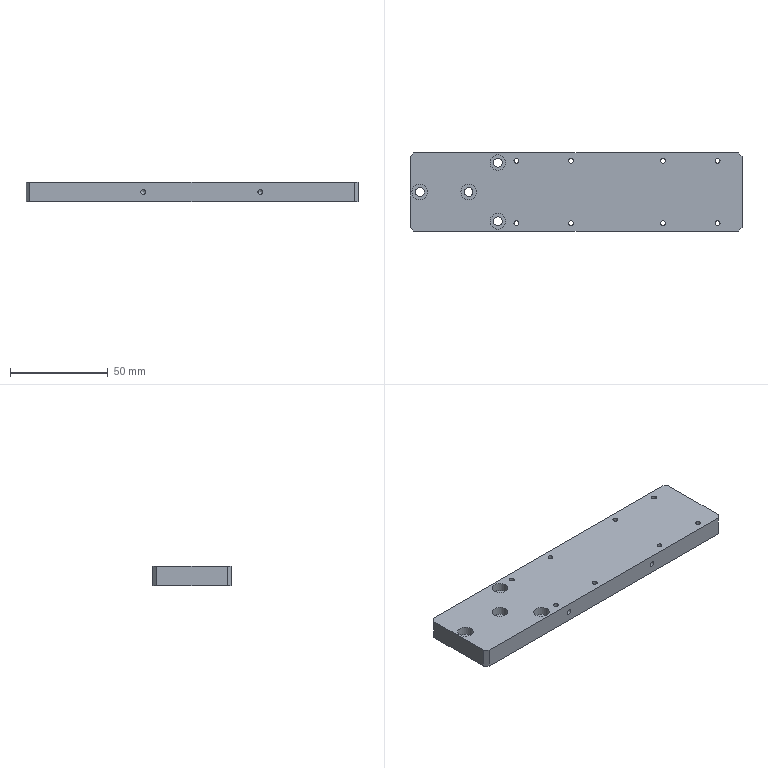Part | NX | 1 solid | 38 faces | box 170 x 40 x 10 mm | volume 66032 mm3 | cylinder 20 | plane 14 | cone 4 | commonest cylinder face diameters 2.5 x10 4.5 x4 8 x4 3.3 x2
STEP:
#1=CARTESIAN_POINT('',(85.,18.,10.));
#2=VERTEX_POINT('',#1);
#3=CARTESIAN_POINT('',(83.,20.,10.));
#4=VERTEX_POINT('',#3);
#5=CARTESIAN_POINT('',(51.5,51.5,10.));
#6=DIRECTION('',(-0.7071,0.7071,0.));
#7=VECTOR('',#6,1000.);
#8=LINE('',#5,#7);
#9=EDGE_CURVE('',#2,#4,#8,.T.);
#10=ORIENTED_EDGE('',*,*,#9,.F.);
#11=CARTESIAN_POINT('',(85.,18.,0.));
#12=VERTEX_POINT('',#11);
#13=CARTESIAN_POINT('',(85.,18.,10.));
#14=DIRECTION('',(0.,0.,1.));
#15=VECTOR('',#14,1000.);
#16=LINE('',#13,#15);
#17=EDGE_CURVE('',#12,#2,#16,.T.);
#18=ORIENTED_EDGE('',*,*,#17,.F.);
#19=CARTESIAN_POINT('',(83.,20.,0.));
#20=VERTEX_POINT('',#19);
#21=CARTESIAN_POINT('',(83.,20.,0.));
#22=DIRECTION('',(0.7071,-0.7071,0.));
#23=VECTOR('',#22,1000.);
#24=LINE('',#21,#23);
#25=EDGE_CURVE('',#20,#12,#24,.T.);
#26=ORIENTED_EDGE('',*,*,#25,.F.);
#27=CARTESIAN_POINT('',(83.,20.,10.));
#28=DIRECTION('',(0.,0.,-1.));
#29=VECTOR('',#28,1000.);
#30=LINE('',#27,#29);
#31=EDGE_CURVE('',#4,#20,#30,.T.);
#32=ORIENTED_EDGE('',*,*,#31,.F.);
#33=EDGE_LOOP('',(#10,#18,#26,#32));
#34=FACE_BOUND('',#33,.T.);
#35=CARTESIAN_POINT('',(83.,20.,10.));
#36=DIRECTION('',(-0.7071,-0.7071,0.));
#37=DIRECTION('',(0.,0.,-1.));
#38=AXIS2_PLACEMENT_3D('',#35,#36,#37);
#39=PLANE('',#38);
#40=ADVANCED_FACE('',(#34),#39,.F.);
#41=CARTESIAN_POINT('',(83.,-20.,10.));
#42=VERTEX_POINT('',#41);
#43=CARTESIAN_POINT('',(85.,-18.,10.));
#44=VERTEX_POINT('',#43);
#45=CARTESIAN_POINT('',(51.5,-51.5,10.));
#46=DIRECTION('',(0.7071,0.7071,0.));
#47=VECTOR('',#46,1000.);
#48=LINE('',#45,#47);
#49=EDGE_CURVE('',#42,#44,#48,.T.);
#50=ORIENTED_EDGE('',*,*,#49,.F.);
#51=CARTESIAN_POINT('',(83.,-20.,0.));
#52=VERTEX_POINT('',#51);
#53=CARTESIAN_POINT('',(83.,-20.,10.));
#54=DIRECTION('',(0.,0.,1.));
#55=VECTOR('',#54,1000.);
#56=LINE('',#53,#55);
#57=EDGE_CURVE('',#52,#42,#56,.T.);
#58=ORIENTED_EDGE('',*,*,#57,.F.);
#59=CARTESIAN_POINT('',(85.,-18.,0.));
#60=VERTEX_POINT('',#59);
#61=CARTESIAN_POINT('',(85.,-18.,0.));
#62=DIRECTION('',(-0.7071,-0.7071,0.));
#63=VECTOR('',#62,1000.);
#64=LINE('',#61,#63);
#65=EDGE_CURVE('',#60,#52,#64,.T.);
#66=ORIENTED_EDGE('',*,*,#65,.F.);
#67=CARTESIAN_POINT('',(85.,-18.,10.));
#68=DIRECTION('',(0.,0.,-1.));
#69=VECTOR('',#68,1000.);
#70=LINE('',#67,#69);
#71=EDGE_CURVE('',#44,#60,#70,.T.);
#72=ORIENTED_EDGE('',*,*,#71,.F.);
#73=EDGE_LOOP('',(#50,#58,#66,#72));
#74=FACE_BOUND('',#73,.T.);
#75=CARTESIAN_POINT('',(85.,-18.,10.));
#76=DIRECTION('',(-0.7071,0.7071,0.));
#77=DIRECTION('',(0.,0.,-1.));
#78=AXIS2_PLACEMENT_3D('',#75,#76,#77);
#79=PLANE('',#78);
#80=ADVANCED_FACE('',(#74),#79,.F.);
#81=CARTESIAN_POINT('',(-85.,-18.,10.));
#82=VERTEX_POINT('',#81);
#83=CARTESIAN_POINT('',(-83.,-20.,10.));
#84=VERTEX_POINT('',#83);
#85=CARTESIAN_POINT('',(-51.5,-51.5,10.));
#86=DIRECTION('',(0.7071,-0.7071,0.));
#87=VECTOR('',#86,1000.);
#88=LINE('',#85,#87);
#89=EDGE_CURVE('',#82,#84,#88,.T.);
#90=ORIENTED_EDGE('',*,*,#89,.F.);
#91=CARTESIAN_POINT('',(-85.,-18.,0.));
#92=VERTEX_POINT('',#91);
#93=CARTESIAN_POINT('',(-85.,-18.,10.));
#94=DIRECTION('',(0.,0.,1.));
#95=VECTOR('',#94,1000.);
#96=LINE('',#93,#95);
#97=EDGE_CURVE('',#92,#82,#96,.T.);
#98=ORIENTED_EDGE('',*,*,#97,.F.);
#99=CARTESIAN_POINT('',(-83.,-20.,0.));
#100=VERTEX_POINT('',#99);
#101=CARTESIAN_POINT('',(-83.,-20.,0.));
#102=DIRECTION('',(-0.7071,0.7071,0.));
#103=VECTOR('',#102,1000.);
#104=LINE('',#101,#103);
#105=EDGE_CURVE('',#100,#92,#104,.T.);
#106=ORIENTED_EDGE('',*,*,#105,.F.);
#107=CARTESIAN_POINT('',(-83.,-20.,10.));
#108=DIRECTION('',(0.,0.,-1.));
#109=VECTOR('',#108,1000.);
#110=LINE('',#107,#109);
#111=EDGE_CURVE('',#84,#100,#110,.T.);
#112=ORIENTED_EDGE('',*,*,#111,.F.);
#113=EDGE_LOOP('',(#90,#98,#106,#112));
#114=FACE_BOUND('',#113,.T.);
#115=CARTESIAN_POINT('',(-83.,-20.,10.));
#116=DIRECTION('',(0.7071,0.7071,0.));
#117=DIRECTION('',(0.,0.,-1.));
#118=AXIS2_PLACEMENT_3D('',#115,#116,#117);
#119=PLANE('',#118);
#120=ADVANCED_FACE('',(#114),#119,.F.);
#121=CARTESIAN_POINT('',(-83.,20.,10.));
#122=VERTEX_POINT('',#121);
#123=CARTESIAN_POINT('',(-85.,18.,10.));
#124=VERTEX_POINT('',#123);
#125=CARTESIAN_POINT('',(-51.5,51.5,10.));
#126=DIRECTION('',(-0.7071,-0.7071,0.));
#127=VECTOR('',#126,1000.);
#128=LINE('',#125,#127);
#129=EDGE_CURVE('',#122,#124,#128,.T.);
#130=ORIENTED_EDGE('',*,*,#129,.F.);
#131=CARTESIAN_POINT('',(-83.,20.,0.));
#132=VERTEX_POINT('',#131);
#133=CARTESIAN_POINT('',(-83.,20.,10.));
#134=DIRECTION('',(0.,0.,1.));
#135=VECTOR('',#134,1000.);
#136=LINE('',#133,#135);
#137=EDGE_CURVE('',#132,#122,#136,.T.);
#138=ORIENTED_EDGE('',*,*,#137,.F.);
#139=CARTESIAN_POINT('',(-85.,18.,0.));
#140=VERTEX_POINT('',#139);
#141=CARTESIAN_POINT('',(-85.,18.,0.));
#142=DIRECTION('',(0.7071,0.7071,0.));
#143=VECTOR('',#142,1000.);
#144=LINE('',#141,#143);
#145=EDGE_CURVE('',#140,#132,#144,.T.);
#146=ORIENTED_EDGE('',*,*,#145,.F.);
#147=CARTESIAN_POINT('',(-85.,18.,10.));
#148=DIRECTION('',(0.,0.,-1.));
#149=VECTOR('',#148,1000.);
#150=LINE('',#147,#149);
#151=EDGE_CURVE('',#124,#140,#150,.T.);
#152=ORIENTED_EDGE('',*,*,#151,.F.);
#153=EDGE_LOOP('',(#130,#138,#146,#152));
#154=FACE_BOUND('',#153,.T.);
#155=CARTESIAN_POINT('',(-85.,18.,10.));
#156=DIRECTION('',(0.7071,-0.7071,0.));
#157=DIRECTION('',(0.,0.,-1.));
#158=AXIS2_PLACEMENT_3D('',#155,#156,#157);
#159=PLANE('',#158);
#160=ADVANCED_FACE('',(#154),#159,.F.);
#161=CARTESIAN_POINT('',(-59.,0.,5.6));
#162=VERTEX_POINT('',#161);
#163=CARTESIAN_POINT('',(-55.,0.,5.6));
#164=DIRECTION('',(0.,0.,1.));
#165=DIRECTION('',(-1.,0.,0.));
#166=AXIS2_PLACEMENT_3D('',#163,#164,#165);
#167=CIRCLE('',#166,4.);
#168=EDGE_CURVE('',#162,#162,#167,.T.);
#169=ORIENTED_EDGE('',*,*,#168,.T.);
#170=EDGE_LOOP('',(#169));
#171=FACE_BOUND('',#170,.T.);
#172=CARTESIAN_POINT('',(-57.25,0.,5.6));
#173=VERTEX_POINT('',#172);
#174=CARTESIAN_POINT('',(-55.,0.,5.6));
#175=DIRECTION('',(0.,0.,1.));
#176=DIRECTION('',(-1.,0.,0.));
#177=AXIS2_PLACEMENT_3D('',#174,#175,#176);
#178=CIRCLE('',#177,2.25);
#179=EDGE_CURVE('',#173,#173,#178,.T.);
#180=ORIENTED_EDGE('',*,*,#179,.F.);
#181=EDGE_LOOP('',(#180));
#182=FACE_BOUND('',#181,.T.);
#183=CARTESIAN_POINT('',(-77.75,0.,5.6));
#184=DIRECTION('',(0.,0.,-1.));
#185=DIRECTION('',(-1.,0.,0.));
#186=AXIS2_PLACEMENT_3D('',#183,#184,#185);
#187=PLANE('',#186);
#188=ADVANCED_FACE('',(#171,#182),#187,.F.);
#189=CARTESIAN_POINT('',(-76.,0.,5.6));
#190=VERTEX_POINT('',#189);
#191=CARTESIAN_POINT('',(-80.,0.,5.6));
#192=DIRECTION('',(0.,0.,1.));
#193=DIRECTION('',(1.,0.,0.));
#194=AXIS2_PLACEMENT_3D('',#191,#192,#193);
#195=CIRCLE('',#194,4.);
#196=EDGE_CURVE('',#190,#190,#195,.T.);
#197=ORIENTED_EDGE('',*,*,#196,.T.);
#198=EDGE_LOOP('',(#197));
#199=FACE_BOUND('',#198,.T.);
#200=CARTESIAN_POINT('',(-77.75,0.,5.6));
#201=VERTEX_POINT('',#200);
#202=CARTESIAN_POINT('',(-80.,0.,5.6));
#203=DIRECTION('',(0.,0.,1.));
#204=DIRECTION('',(1.,0.,0.));
#205=AXIS2_PLACEMENT_3D('',#202,#203,#204);
#206=CIRCLE('',#205,2.25);
#207=EDGE_CURVE('',#201,#201,#206,.T.);
#208=ORIENTED_EDGE('',*,*,#207,.F.);
#209=EDGE_LOOP('',(#208));
#210=FACE_BOUND('',#209,.T.);
#211=CARTESIAN_POINT('',(-77.75,0.,5.6));
#212=DIRECTION('',(0.,0.,-1.));
#213=DIRECTION('',(-1.,0.,0.));
#214=AXIS2_PLACEMENT_3D('',#211,#212,#213);
#215=PLANE('',#214);
#216=ADVANCED_FACE('',(#199,#210),#215,.F.);
#217=CARTESIAN_POINT('',(-44.,15.,5.6));
#218=VERTEX_POINT('',#217);
#219=CARTESIAN_POINT('',(-40.,15.,5.6));
#220=DIRECTION('',(0.,0.,1.));
#221=DIRECTION('',(-1.,0.,0.));
#222=AXIS2_PLACEMENT_3D('',#219,#220,#221);
#223=CIRCLE('',#222,4.);
#224=EDGE_CURVE('',#218,#218,#223,.T.);
#225=ORIENTED_EDGE('',*,*,#224,.T.);
#226=EDGE_LOOP('',(#225));
#227=FACE_BOUND('',#226,.T.);
#228=CARTESIAN_POINT('',(-42.25,15.,5.6));
#229=VERTEX_POINT('',#228);
#230=CARTESIAN_POINT('',(-40.,15.,5.6));
#231=DIRECTION('',(0.,0.,1.));
#232=DIRECTION('',(-1.,0.,0.));
#233=AXIS2_PLACEMENT_3D('',#230,#231,#232);
#234=CIRCLE('',#233,2.25);
#235=EDGE_CURVE('',#229,#229,#234,.T.);
#236=ORIENTED_EDGE('',*,*,#235,.F.);
#237=EDGE_LOOP('',(#236));
#238=FACE_BOUND('',#237,.T.);
#239=CARTESIAN_POINT('',(-77.75,0.,5.6));
#240=DIRECTION('',(0.,0.,-1.));
#241=DIRECTION('',(-1.,0.,0.));
#242=AXIS2_PLACEMENT_3D('',#239,#240,#241);
#243=PLANE('',#242);
#244=ADVANCED_FACE('',(#227,#238),#243,.F.);
#245=CARTESIAN_POINT('',(-44.,-15.,5.6));
#246=VERTEX_POINT('',#245);
#247=CARTESIAN_POINT('',(-40.,-15.,5.6));
#248=DIRECTION('',(0.,0.,1.));
#249=DIRECTION('',(-1.,0.,0.));
#250=AXIS2_PLACEMENT_3D('',#247,#248,#249);
#251=CIRCLE('',#250,4.);
#252=EDGE_CURVE('',#246,#246,#251,.T.);
#253=ORIENTED_EDGE('',*,*,#252,.T.);
#254=EDGE_LOOP('',(#253));
#255=FACE_BOUND('',#254,.T.);
#256=CARTESIAN_POINT('',(-42.25,-15.,5.6));
#257=VERTEX_POINT('',#256);
#258=CARTESIAN_POINT('',(-40.,-15.,5.6));
#259=DIRECTION('',(0.,0.,1.));
#260=DIRECTION('',(-1.,0.,0.));
#261=AXIS2_PLACEMENT_3D('',#258,#259,#260);
#262=CIRCLE('',#261,2.25);
#263=EDGE_CURVE('',#257,#257,#262,.T.);
#264=ORIENTED_EDGE('',*,*,#263,.F.);
#265=EDGE_LOOP('',(#264));
#266=FACE_BOUND('',#265,.T.);
#267=CARTESIAN_POINT('',(-77.75,0.,5.6));
#268=DIRECTION('',(0.,0.,-1.));
#269=DIRECTION('',(-1.,0.,0.));
#270=AXIS2_PLACEMENT_3D('',#267,#268,#269);
#271=PLANE('',#270);
#272=ADVANCED_FACE('',(#255,#266),#271,.F.);
#273=CARTESIAN_POINT('',(-85.,20.,0.));
#274=DIRECTION('',(0.,-1.,0.));
#275=VECTOR('',#274,1000.);
#276=LINE('',#273,#275);
#277=EDGE_CURVE('',#140,#92,#276,.T.);
#278=ORIENTED_EDGE('',*,*,#277,.F.);
#279=ORIENTED_EDGE('',*,*,#145,.T.);
#280=CARTESIAN_POINT('',(-85.,20.,0.));
#281=DIRECTION('',(-1.,0.,0.));
#282=VECTOR('',#281,1000.);
#283=LINE('',#280,#282);
#284=EDGE_CURVE('',#20,#132,#283,.T.);
#285=ORIENTED_EDGE('',*,*,#284,.F.);
#286=ORIENTED_EDGE('',*,*,#25,.T.);
#287=CARTESIAN_POINT('',(85.,20.,0.));
#288=DIRECTION('',(0.,1.,0.));
#289=VECTOR('',#288,1000.);
#290=LINE('',#287,#289);
#291=EDGE_CURVE('',#60,#12,#290,.T.);
#292=ORIENTED_EDGE('',*,*,#291,.F.);
#293=ORIENTED_EDGE('',*,*,#65,.T.);
#294=CARTESIAN_POINT('',(-85.,-20.,0.));
#295=DIRECTION('',(1.,0.,0.));
#296=VECTOR('',#295,1000.);
#297=LINE('',#294,#296);
#298=EDGE_CURVE('',#100,#52,#297,.T.);
#299=ORIENTED_EDGE('',*,*,#298,.F.);
#300=ORIENTED_EDGE('',*,*,#105,.T.);
#301=EDGE_LOOP('',(#278,#279,#285,#286,#292,#293,#299,#300));
#302=FACE_BOUND('',#301,.T.);
#303=CARTESIAN_POINT('',(45.75,16.,0.));
#304=VERTEX_POINT('',#303);
#305=CARTESIAN_POINT('',(44.5,16.,0.));
#306=DIRECTION('',(0.,0.,1.));
#307=DIRECTION('',(1.,0.,0.));
#308=AXIS2_PLACEMENT_3D('',#305,#306,#307);
#309=CIRCLE('',#308,1.25);
#310=EDGE_CURVE('',#304,#304,#309,.T.);
#311=ORIENTED_EDGE('',*,*,#310,.T.);
#312=EDGE_LOOP('',(#311));
#313=FACE_BOUND('',#312,.T.);
#314=CARTESIAN_POINT('',(-29.25,16.,0.));
#315=VERTEX_POINT('',#314);
#316=CARTESIAN_POINT('',(-30.5,16.,0.));
#317=DIRECTION('',(0.,0.,1.));
#318=DIRECTION('',(1.,0.,0.));
#319=AXIS2_PLACEMENT_3D('',#316,#317,#318);
#320=CIRCLE('',#319,1.25);
#321=EDGE_CURVE('',#315,#315,#320,.T.);
#322=ORIENTED_EDGE('',*,*,#321,.T.);
#323=EDGE_LOOP('',(#322));
#324=FACE_BOUND('',#323,.T.);
#325=CARTESIAN_POINT('',(-29.25,-16.,0.));
#326=VERTEX_POINT('',#325);
#327=CARTESIAN_POINT('',(-30.5,-16.,0.));
#328=DIRECTION('',(0.,0.,1.));
#329=DIRECTION('',(1.,0.,0.));
#330=AXIS2_PLACEMENT_3D('',#327,#328,#329);
#331=CIRCLE('',#330,1.25);
#332=EDGE_CURVE('',#326,#326,#331,.T.);
#333=ORIENTED_EDGE('',*,*,#332,.T.);
#334=EDGE_LOOP('',(#333));
#335=FACE_BOUND('',#334,.T.);
#336=CARTESIAN_POINT('',(45.75,-16.,0.));
#337=VERTEX_POINT('',#336);
#338=CARTESIAN_POINT('',(44.5,-16.,0.));
#339=DIRECTION('',(0.,0.,1.));
#340=DIRECTION('',(1.,0.,0.));
#341=AXIS2_PLACEMENT_3D('',#338,#339,#340);
#342=CIRCLE('',#341,1.25);
#343=EDGE_CURVE('',#337,#337,#342,.T.);
#344=ORIENTED_EDGE('',*,*,#343,.T.);
#345=EDGE_LOOP('',(#344));
#346=FACE_BOUND('',#345,.T.);
#347=CARTESIAN_POINT('',(-1.25,-16.,0.));
#348=VERTEX_POINT('',#347);
#349=CARTESIAN_POINT('',(-2.5,-16.,0.));
#350=DIRECTION('',(0.,0.,1.));
#351=DIRECTION('',(1.,0.,0.));
#352=AXIS2_PLACEMENT_3D('',#349,#350,#351);
#353=CIRCLE('',#352,1.25);
#354=EDGE_CURVE('',#348,#348,#353,.T.);
#355=ORIENTED_EDGE('',*,*,#354,.T.);
#356=EDGE_LOOP('',(#355));
#357=FACE_BOUND('',#356,.T.);
#358=CARTESIAN_POINT('',(-1.25,16.,0.));
#359=VERTEX_POINT('',#358);
#360=CARTESIAN_POINT('',(-2.5,16.,0.));
#361=DIRECTION('',(0.,0.,1.));
#362=DIRECTION('',(1.,0.,0.));
#363=AXIS2_PLACEMENT_3D('',#360,#361,#362);
#364=CIRCLE('',#363,1.25);
#365=EDGE_CURVE('',#359,#359,#364,.T.);
#366=ORIENTED_EDGE('',*,*,#365,.T.);
#367=EDGE_LOOP('',(#366));
#368=FACE_BOUND('',#367,.T.);
#369=CARTESIAN_POINT('',(73.75,-16.,0.));
#370=VERTEX_POINT('',#369);
#371=CARTESIAN_POINT('',(72.5,-16.,0.));
#372=DIRECTION('',(0.,0.,1.));
#373=DIRECTION('',(1.,0.,0.));
#374=AXIS2_PLACEMENT_3D('',#371,#372,#373);
#375=CIRCLE('',#374,1.25);
#376=EDGE_CURVE('',#370,#370,#375,.T.);
#377=ORIENTED_EDGE('',*,*,#376,.T.);
#378=EDGE_LOOP('',(#377));
#379=FACE_BOUND('',#378,.T.);
#380=CARTESIAN_POINT('',(73.75,16.,0.));
#381=VERTEX_POINT('',#380);
#382=CARTESIAN_POINT('',(72.5,16.,0.));
#383=DIRECTION('',(0.,0.,1.));
#384=DIRECTION('',(1.,0.,0.));
#385=AXIS2_PLACEMENT_3D('',#382,#383,#384);
#386=CIRCLE('',#385,1.25);
#387=EDGE_CURVE('',#381,#381,#386,.T.);
#388=ORIENTED_EDGE('',*,*,#387,.T.);
#389=EDGE_LOOP('',(#388));
#390=FACE_BOUND('',#389,.T.);
#391=CARTESIAN_POINT('',(-37.75,-15.,0.));
#392=VERTEX_POINT('',#391);
#393=CARTESIAN_POINT('',(-40.,-15.,0.));
#394=DIRECTION('',(0.,0.,1.));
#395=DIRECTION('',(1.,0.,0.));
#396=AXIS2_PLACEMENT_3D('',#393,#394,#395);
#397=CIRCLE('',#396,2.25);
#398=EDGE_CURVE('',#392,#392,#397,.T.);
#399=ORIENTED_EDGE('',*,*,#398,.T.);
#400=EDGE_LOOP('',(#399));
#401=FACE_BOUND('',#400,.T.);
#402=CARTESIAN_POINT('',(-37.75,15.,0.));
#403=VERTEX_POINT('',#402);
#404=CARTESIAN_POINT('',(-40.,15.,0.));
#405=DIRECTION('',(0.,0.,1.));
#406=DIRECTION('',(1.,0.,0.));
#407=AXIS2_PLACEMENT_3D('',#404,#405,#406);
#408=CIRCLE('',#407,2.25);
#409=EDGE_CURVE('',#403,#403,#408,.T.);
#410=ORIENTED_EDGE('',*,*,#409,.T.);
#411=EDGE_LOOP('',(#410));
#412=FACE_BOUND('',#411,.T.);
#413=CARTESIAN_POINT('',(-77.75,0.,0.));
#414=VERTEX_POINT('',#413);
#415=CARTESIAN_POINT('',(-80.,0.,0.));
#416=DIRECTION('',(0.,0.,1.));
#417=DIRECTION('',(1.,0.,0.));
#418=AXIS2_PLACEMENT_3D('',#415,#416,#417);
#419=CIRCLE('',#418,2.25);
#420=EDGE_CURVE('',#414,#414,#419,.T.);
#421=ORIENTED_EDGE('',*,*,#420,.T.);
#422=EDGE_LOOP('',(#421));
#423=FACE_BOUND('',#422,.T.);
#424=CARTESIAN_POINT('',(-52.75,0.,0.));
#425=VERTEX_POINT('',#424);
#426=CARTESIAN_POINT('',(-55.,0.,0.));
#427=DIRECTION('',(0.,0.,1.));
#428=DIRECTION('',(1.,0.,0.));
#429=AXIS2_PLACEMENT_3D('',#426,#427,#428);
#430=CIRCLE('',#429,2.25);
#431=EDGE_CURVE('',#425,#425,#430,.T.);
#432=ORIENTED_EDGE('',*,*,#431,.T.);
#433=EDGE_LOOP('',(#432));
#434=FACE_BOUND('',#433,.T.);
#435=CARTESIAN_POINT('',(0.,0.,0.));
#436=DIRECTION('',(0.,0.,1.));
#437=DIRECTION('',(1.,0.,0.));
#438=AXIS2_PLACEMENT_3D('',#435,#436,#437);
#439=PLANE('',#438);
#440=ADVANCED_FACE('',(#302,#313,#324,#335,#346,#357,#368,#379,#390,#401,#412,#423,#434),#439,.F.);
#441=CARTESIAN_POINT('',(-85.,20.,10.));
#442=DIRECTION('',(-1.,0.,0.));
#443=VECTOR('',#442,1000.);
#444=LINE('',#441,#443);
#445=EDGE_CURVE('',#4,#122,#444,.T.);
#446=ORIENTED_EDGE('',*,*,#445,.T.);
#447=ORIENTED_EDGE('',*,*,#129,.T.);
#448=CARTESIAN_POINT('',(-85.,20.,10.));
#449=DIRECTION('',(0.,-1.,0.));
#450=VECTOR('',#449,1000.);
#451=LINE('',#448,#450);
#452=EDGE_CURVE('',#124,#82,#451,.T.);
#453=ORIENTED_EDGE('',*,*,#452,.T.);
#454=ORIENTED_EDGE('',*,*,#89,.T.);
#455=CARTESIAN_POINT('',(-85.,-20.,10.));
#456=DIRECTION('',(1.,0.,0.));
#457=VECTOR('',#456,1000.);
#458=LINE('',#455,#457);
#459=EDGE_CURVE('',#84,#42,#458,.T.);
#460=ORIENTED_EDGE('',*,*,#459,.T.);
#461=ORIENTED_EDGE('',*,*,#49,.T.);
#462=CARTESIAN_POINT('',(85.,20.,10.));
#463=DIRECTION('',(0.,1.,0.));
#464=VECTOR('',#463,1000.);
#465=LINE('',#462,#464);
#466=EDGE_CURVE('',#44,#2,#465,.T.);
#467=ORIENTED_EDGE('',*,*,#466,.T.);
#468=ORIENTED_EDGE('',*,*,#9,.T.);
#469=EDGE_LOOP('',(#446,#447,#453,#454,#460,#461,#467,#468));
#470=FACE_BOUND('',#469,.T.);
#471=CARTESIAN_POINT('',(45.75,16.,10.));
#472=VERTEX_POINT('',#471);
#473=CARTESIAN_POINT('',(44.5,16.,10.));
#474=DIRECTION('',(0.,0.,1.));
#475=DIRECTION('',(1.,0.,0.));
#476=AXIS2_PLACEMENT_3D('',#473,#474,#475);
#477=CIRCLE('',#476,1.25);
#478=EDGE_CURVE('',#472,#472,#477,.T.);
#479=ORIENTED_EDGE('',*,*,#478,.F.);
#480=EDGE_LOOP('',(#479));
#481=FACE_BOUND('',#480,.T.);
#482=CARTESIAN_POINT('',(-29.25,16.,10.));
#483=VERTEX_POINT('',#482);
#484=CARTESIAN_POINT('',(-30.5,16.,10.));
#485=DIRECTION('',(0.,0.,1.));
#486=DIRECTION('',(1.,0.,0.));
#487=AXIS2_PLACEMENT_3D('',#484,#485,#486);
#488=CIRCLE('',#487,1.25);
#489=EDGE_CURVE('',#483,#483,#488,.T.);
#490=ORIENTED_EDGE('',*,*,#489,.F.);
#491=EDGE_LOOP('',(#490));
#492=FACE_BOUND('',#491,.T.);
#493=CARTESIAN_POINT('',(-29.25,-16.,10.));
#494=VERTEX_POINT('',#493);
#495=CARTESIAN_POINT('',(-30.5,-16.,10.));
#496=DIRECTION('',(0.,0.,1.));
#497=DIRECTION('',(1.,0.,0.));
#498=AXIS2_PLACEMENT_3D('',#495,#496,#497);
#499=CIRCLE('',#498,1.25);
#500=EDGE_CURVE('',#494,#494,#499,.T.);
#501=ORIENTED_EDGE('',*,*,#500,.F.);
#502=EDGE_LOOP('',(#501));
#503=FACE_BOUND('',#502,.T.);
#504=CARTESIAN_POINT('',(45.75,-16.,10.));
#505=VERTEX_POINT('',#504);
#506=CARTESIAN_POINT('',(44.5,-16.,10.));
#507=DIRECTION('',(0.,0.,1.));
#508=DIRECTION('',(1.,0.,0.));
#509=AXIS2_PLACEMENT_3D('',#506,#507,#508);
#510=CIRCLE('',#509,1.25);
#511=EDGE_CURVE('',#505,#505,#510,.T.);
#512=ORIENTED_EDGE('',*,*,#511,.F.);
#513=EDGE_LOOP('',(#512));
#514=FACE_BOUND('',#513,.T.);
#515=CARTESIAN_POINT('',(-1.25,-16.,10.));
#516=VERTEX_POINT('',#515);
#517=CARTESIAN_POINT('',(-2.5,-16.,10.));
#518=DIRECTION('',(0.,0.,1.));
#519=DIRECTION('',(1.,0.,0.));
#520=AXIS2_PLACEMENT_3D('',#517,#518,#519);
#521=CIRCLE('',#520,1.25);
#522=EDGE_CURVE('',#516,#516,#521,.T.);
#523=ORIENTED_EDGE('',*,*,#522,.F.);
#524=EDGE_LOOP('',(#523));
#525=FACE_BOUND('',#524,.T.);
#526=CARTESIAN_POINT('',(-1.25,16.,10.));
#527=VERTEX_POINT('',#526);
#528=CARTESIAN_POINT('',(-2.5,16.,10.));
#529=DIRECTION('',(0.,0.,1.));
#530=DIRECTION('',(1.,0.,0.));
#531=AXIS2_PLACEMENT_3D('',#528,#529,#530);
#532=CIRCLE('',#531,1.25);
#533=EDGE_CURVE('',#527,#527,#532,.T.);
#534=ORIENTED_EDGE('',*,*,#533,.F.);
#535=EDGE_LOOP('',(#534));
#536=FACE_BOUND('',#535,.T.);
#537=CARTESIAN_POINT('',(73.75,-16.,10.));
#538=VERTEX_POINT('',#537);
#539=CARTESIAN_POINT('',(72.5,-16.,10.));
#540=DIRECTION('',(0.,0.,1.));
#541=DIRECTION('',(1.,0.,0.));
#542=AXIS2_PLACEMENT_3D('',#539,#540,#541);
#543=CIRCLE('',#542,1.25);
#544=EDGE_CURVE('',#538,#538,#543,.T.);
#545=ORIENTED_EDGE('',*,*,#544,.F.);
#546=EDGE_LOOP('',(#545));
#547=FACE_BOUND('',#546,.T.);
#548=CARTESIAN_POINT('',(73.75,16.,10.));
#549=VERTEX_POINT('',#548);
#550=CARTESIAN_POINT('',(72.5,16.,10.));
#551=DIRECTION('',(0.,0.,1.));
#552=DIRECTION('',(1.,0.,0.));
#553=AXIS2_PLACEMENT_3D('',#550,#551,#552);
#554=CIRCLE('',#553,1.25);
#555=EDGE_CURVE('',#549,#549,#554,.T.);
#556=ORIENTED_EDGE('',*,*,#555,.F.);
#557=EDGE_LOOP('',(#556));
#558=FACE_BOUND('',#557,.T.);
#559=CARTESIAN_POINT('',(-36.,-15.,10.));
#560=VERTEX_POINT('',#559);
#561=CARTESIAN_POINT('',(-40.,-15.,10.));
#562=DIRECTION('',(0.,0.,1.));
#563=DIRECTION('',(1.,0.,0.));
#564=AXIS2_PLACEMENT_3D('',#561,#562,#563);
#565=CIRCLE('',#564,4.);
#566=EDGE_CURVE('',#560,#560,#565,.T.);
#567=ORIENTED_EDGE('',*,*,#566,.F.);
#568=EDGE_LOOP('',(#567));
#569=FACE_BOUND('',#568,.T.);
#570=CARTESIAN_POINT('',(-36.,15.,10.));
#571=VERTEX_POINT('',#570);
#572=CARTESIAN_POINT('',(-40.,15.,10.));
#573=DIRECTION('',(0.,0.,1.));
#574=DIRECTION('',(1.,0.,0.));
#575=AXIS2_PLACEMENT_3D('',#572,#573,#574);
#576=CIRCLE('',#575,4.);
#577=EDGE_CURVE('',#571,#571,#576,.T.);
#578=ORIENTED_EDGE('',*,*,#577,.F.);
#579=EDGE_LOOP('',(#578));
#580=FACE_BOUND('',#579,.T.);
#581=CARTESIAN_POINT('',(-76.,0.,10.));
#582=VERTEX_POINT('',#581);
#583=CARTESIAN_POINT('',(-80.,0.,10.));
#584=DIRECTION('',(0.,0.,1.));
#585=DIRECTION('',(1.,0.,0.));
#586=AXIS2_PLACEMENT_3D('',#583,#584,#585);
#587=CIRCLE('',#586,4.);
#588=EDGE_CURVE('',#582,#582,#587,.T.);
#589=ORIENTED_EDGE('',*,*,#588,.F.);
#590=EDGE_LOOP('',(#589));
#591=FACE_BOUND('',#590,.T.);
#592=CARTESIAN_POINT('',(-51.,0.,10.));
#593=VERTEX_POINT('',#592);
#594=CARTESIAN_POINT('',(-55.,0.,10.));
#595=DIRECTION('',(0.,0.,1.));
#596=DIRECTION('',(1.,0.,0.));
#597=AXIS2_PLACEMENT_3D('',#594,#595,#596);
#598=CIRCLE('',#597,4.);
#599=EDGE_CURVE('',#593,#593,#598,.T.);
#600=ORIENTED_EDGE('',*,*,#599,.F.);
#601=EDGE_LOOP('',(#600));
#602=FACE_BOUND('',#601,.T.);
#603=CARTESIAN_POINT('',(0.,0.,10.));
#604=DIRECTION('',(0.,0.,1.));
#605=DIRECTION('',(1.,0.,0.));
#606=AXIS2_PLACEMENT_3D('',#603,#604,#605);
#607=PLANE('',#606);
#608=ADVANCED_FACE('',(#470,#481,#492,#503,#514,#525,#536,#547,#558,#569,#580,#591,#602),#607,.T.);
#609=ORIENTED_EDGE('',*,*,#459,.F.);
#610=ORIENTED_EDGE('',*,*,#111,.T.);
#611=ORIENTED_EDGE('',*,*,#298,.T.);
#612=ORIENTED_EDGE('',*,*,#57,.T.);
#613=EDGE_LOOP('',(#609,#610,#611,#612));
#614=FACE_BOUND('',#613,.T.);
#615=CARTESIAN_POINT('',(35.,-20.,3.75));
#616=VERTEX_POINT('',#615);
#617=CARTESIAN_POINT('',(35.,-20.,5.));
#618=DIRECTION('',(0.,-1.,0.));
#619=DIRECTION('',(0.,0.,-1.));
#620=AXIS2_PLACEMENT_3D('',#617,#618,#619);
#621=CIRCLE('',#620,1.25);
#622=EDGE_CURVE('',#616,#616,#621,.T.);
#623=ORIENTED_EDGE('',*,*,#622,.F.);
#624=EDGE_LOOP('',(#623));
#625=FACE_BOUND('',#624,.T.);
#626=CARTESIAN_POINT('',(-25.,-20.,3.75));
#627=VERTEX_POINT('',#626);
#628=CARTESIAN_POINT('',(-25.,-20.,5.));
#629=DIRECTION('',(0.,-1.,0.));
#630=DIRECTION('',(0.,0.,-1.));
#631=AXIS2_PLACEMENT_3D('',#628,#629,#630);
#632=CIRCLE('',#631,1.25);
#633=EDGE_CURVE('',#627,#627,#632,.T.);
#634=ORIENTED_EDGE('',*,*,#633,.F.);
#635=EDGE_LOOP('',(#634));
#636=FACE_BOUND('',#635,.T.);
#637=CARTESIAN_POINT('',(-85.,-20.,10.));
#638=DIRECTION('',(0.,1.,0.));
#639=DIRECTION('',(0.,0.,1.));
#640=AXIS2_PLACEMENT_3D('',#637,#638,#639);
#641=PLANE('',#640);
#642=ADVANCED_FACE('',(#614,#625,#636),#641,.F.);
#643=ORIENTED_EDGE('',*,*,#452,.F.);
#644=ORIENTED_EDGE('',*,*,#151,.T.);
#645=ORIENTED_EDGE('',*,*,#277,.T.);
#646=ORIENTED_EDGE('',*,*,#97,.T.);
#647=EDGE_LOOP('',(#643,#644,#645,#646));
#648=FACE_BOUND('',#647,.T.);
#649=CARTESIAN_POINT('',(-85.,20.,10.));
#650=DIRECTION('',(1.,0.,0.));
#651=DIRECTION('',(0.,0.,-1.));
#652=AXIS2_PLACEMENT_3D('',#649,#650,#651);
#653=PLANE('',#652);
#654=ADVANCED_FACE('',(#648),#653,.F.);
#655=ORIENTED_EDGE('',*,*,#284,.T.);
#656=ORIENTED_EDGE('',*,*,#137,.T.);
#657=ORIENTED_EDGE('',*,*,#445,.F.);
#658=ORIENTED_EDGE('',*,*,#31,.T.);
#659=EDGE_LOOP('',(#655,#656,#657,#658));
#660=FACE_BOUND('',#659,.T.);
#661=CARTESIAN_POINT('',(-56.,20.,6.65));
#662=VERTEX_POINT('',#661);
#663=CARTESIAN_POINT('',(-56.,20.,5.));
#664=DIRECTION('',(0.,1.,0.));
#665=DIRECTION('',(0.,0.,1.));
#666=AXIS2_PLACEMENT_3D('',#663,#664,#665);
#667=CIRCLE('',#666,1.65);
#668=EDGE_CURVE('',#662,#662,#667,.T.);
#669=ORIENTED_EDGE('',*,*,#668,.F.);
#670=EDGE_LOOP('',(#669));
#671=FACE_BOUND('',#670,.T.);
#672=CARTESIAN_POINT('',(-69.,20.,6.65));
#673=VERTEX_POINT('',#672);
#674=CARTESIAN_POINT('',(-69.,20.,5.));
#675=DIRECTION('',(0.,1.,0.));
#676=DIRECTION('',(0.,0.,1.));
#677=AXIS2_PLACEMENT_3D('',#674,#675,#676);
#678=CIRCLE('',#677,1.65);
#679=EDGE_CURVE('',#673,#673,#678,.T.);
#680=ORIENTED_EDGE('',*,*,#679,.F.);
#681=EDGE_LOOP('',(#680));
#682=FACE_BOUND('',#681,.T.);
#683=CARTESIAN_POINT('',(-85.,20.,10.));
#684=DIRECTION('',(0.,-1.,0.));
#685=DIRECTION('',(0.,0.,-1.));
#686=AXIS2_PLACEMENT_3D('',#683,#684,#685);
#687=PLANE('',#686);
#688=ADVANCED_FACE('',(#660,#671,#682),#687,.F.);
#689=ORIENTED_EDGE('',*,*,#466,.F.);
#690=ORIENTED_EDGE('',*,*,#71,.T.);
#691=ORIENTED_EDGE('',*,*,#291,.T.);
#692=ORIENTED_EDGE('',*,*,#17,.T.);
#693=EDGE_LOOP('',(#689,#690,#691,#692));
#694=FACE_BOUND('',#693,.T.);
#695=CARTESIAN_POINT('',(85.,20.,10.));
#696=DIRECTION('',(-1.,0.,0.));
#697=DIRECTION('',(0.,0.,1.));
#698=AXIS2_PLACEMENT_3D('',#695,#696,#697);
#699=PLANE('',#698);
#700=ADVANCED_FACE('',(#694),#699,.F.);
#701=ORIENTED_EDGE('',*,*,#310,.F.);
#702=EDGE_LOOP('',(#701));
#703=FACE_BOUND('',#702,.T.);
#704=ORIENTED_EDGE('',*,*,#478,.T.);
#705=EDGE_LOOP('',(#704));
#706=FACE_BOUND('',#705,.T.);
#707=CARTESIAN_POINT('',(44.5,16.,10.));
#708=DIRECTION('',(0.,0.,1.));
#709=DIRECTION('',(1.,0.,0.));
#710=AXIS2_PLACEMENT_3D('',#707,#708,#709);
#711=CYLINDRICAL_SURFACE('',#710,1.25);
#712=ADVANCED_FACE('',(#703,#706),#711,.F.);
#713=ORIENTED_EDGE('',*,*,#321,.F.);
#714=EDGE_LOOP('',(#713));
#715=FACE_BOUND('',#714,.T.);
#716=ORIENTED_EDGE('',*,*,#489,.T.);
#717=EDGE_LOOP('',(#716));
#718=FACE_BOUND('',#717,.T.);
#719=CARTESIAN_POINT('',(-30.5,16.,10.));
#720=DIRECTION('',(0.,0.,1.));
#721=DIRECTION('',(1.,0.,0.));
#722=AXIS2_PLACEMENT_3D('',#719,#720,#721);
#723=CYLINDRICAL_SURFACE('',#722,1.25);
#724=ADVANCED_FACE('',(#715,#718),#723,.F.);
#725=ORIENTED_EDGE('',*,*,#332,.F.);
#726=EDGE_LOOP('',(#725));
#727=FACE_BOUND('',#726,.T.);
#728=ORIENTED_EDGE('',*,*,#500,.T.);
#729=EDGE_LOOP('',(#728));
#730=FACE_BOUND('',#729,.T.);
#731=CARTESIAN_POINT('',(-30.5,-16.,10.));
#732=DIRECTION('',(0.,0.,1.));
#733=DIRECTION('',(1.,0.,0.));
#734=AXIS2_PLACEMENT_3D('',#731,#732,#733);
#735=CYLINDRICAL_SURFACE('',#734,1.25);
#736=ADVANCED_FACE('',(#727,#730),#735,.F.);
#737=ORIENTED_EDGE('',*,*,#343,.F.);
#738=EDGE_LOOP('',(#737));
#739=FACE_BOUND('',#738,.T.);
#740=ORIENTED_EDGE('',*,*,#511,.T.);
#741=EDGE_LOOP('',(#740));
#742=FACE_BOUND('',#741,.T.);
#743=CARTESIAN_POINT('',(44.5,-16.,10.));
#744=DIRECTION('',(0.,0.,1.));
#745=DIRECTION('',(1.,0.,0.));
#746=AXIS2_PLACEMENT_3D('',#743,#744,#745);
#747=CYLINDRICAL_SURFACE('',#746,1.25);
#748=ADVANCED_FACE('',(#739,#742),#747,.F.);
#749=ORIENTED_EDGE('',*,*,#354,.F.);
#750=EDGE_LOOP('',(#749));
#751=FACE_BOUND('',#750,.T.);
#752=ORIENTED_EDGE('',*,*,#522,.T.);
#753=EDGE_LOOP('',(#752));
#754=FACE_BOUND('',#753,.T.);
#755=CARTESIAN_POINT('',(-2.5,-16.,10.));
#756=DIRECTION('',(0.,0.,1.));
#757=DIRECTION('',(1.,0.,0.));
#758=AXIS2_PLACEMENT_3D('',#755,#756,#757);
#759=CYLINDRICAL_SURFACE('',#758,1.25);
#760=ADVANCED_FACE('',(#751,#754),#759,.F.);
#761=ORIENTED_EDGE('',*,*,#365,.F.);
#762=EDGE_LOOP('',(#761));
#763=FACE_BOUND('',#762,.T.);
#764=ORIENTED_EDGE('',*,*,#533,.T.);
#765=EDGE_LOOP('',(#764));
#766=FACE_BOUND('',#765,.T.);
#767=CARTESIAN_POINT('',(-2.5,16.,10.));
#768=DIRECTION('',(0.,0.,1.));
#769=DIRECTION('',(1.,0.,0.));
#770=AXIS2_PLACEMENT_3D('',#767,#768,#769);
#771=CYLINDRICAL_SURFACE('',#770,1.25);
#772=ADVANCED_FACE('',(#763,#766),#771,.F.);
#773=ORIENTED_EDGE('',*,*,#376,.F.);
#774=EDGE_LOOP('',(#773));
#775=FACE_BOUND('',#774,.T.);
#776=ORIENTED_EDGE('',*,*,#544,.T.);
#777=EDGE_LOOP('',(#776));
#778=FACE_BOUND('',#777,.T.);
#779=CARTESIAN_POINT('',(72.5,-16.,10.));
#780=DIRECTION('',(0.,0.,1.));
#781=DIRECTION('',(1.,0.,0.));
#782=AXIS2_PLACEMENT_3D('',#779,#780,#781);
#783=CYLINDRICAL_SURFACE('',#782,1.25);
#784=ADVANCED_FACE('',(#775,#778),#783,.F.);
#785=ORIENTED_EDGE('',*,*,#387,.F.);
#786=EDGE_LOOP('',(#785));
#787=FACE_BOUND('',#786,.T.);
#788=ORIENTED_EDGE('',*,*,#555,.T.);
#789=EDGE_LOOP('',(#788));
#790=FACE_BOUND('',#789,.T.);
#791=CARTESIAN_POINT('',(72.5,16.,10.));
#792=DIRECTION('',(0.,0.,1.));
#793=DIRECTION('',(1.,0.,0.));
#794=AXIS2_PLACEMENT_3D('',#791,#792,#793);
#795=CYLINDRICAL_SURFACE('',#794,1.25);
#796=ADVANCED_FACE('',(#787,#790),#795,.F.);
#797=ORIENTED_EDGE('',*,*,#398,.F.);
#798=EDGE_LOOP('',(#797));
#799=FACE_BOUND('',#798,.T.);
#800=ORIENTED_EDGE('',*,*,#263,.T.);
#801=EDGE_LOOP('',(#800));
#802=FACE_BOUND('',#801,.T.);
#803=CARTESIAN_POINT('',(-40.,-15.,10.));
#804=DIRECTION('',(0.,0.,1.));
#805=DIRECTION('',(1.,0.,0.));
#806=AXIS2_PLACEMENT_3D('',#803,#804,#805);
#807=CYLINDRICAL_SURFACE('',#806,2.25);
#808=ADVANCED_FACE('',(#799,#802),#807,.F.);
#809=ORIENTED_EDGE('',*,*,#252,.F.);
#810=EDGE_LOOP('',(#809));
#811=FACE_BOUND('',#810,.T.);
#812=ORIENTED_EDGE('',*,*,#566,.T.);
#813=EDGE_LOOP('',(#812));
#814=FACE_BOUND('',#813,.T.);
#815=CARTESIAN_POINT('',(-40.,-15.,10.));
#816=DIRECTION('',(0.,0.,1.));
#817=DIRECTION('',(1.,0.,0.));
#818=AXIS2_PLACEMENT_3D('',#815,#816,#817);
#819=CYLINDRICAL_SURFACE('',#818,4.);
#820=ADVANCED_FACE('',(#811,#814),#819,.F.);
#821=ORIENTED_EDGE('',*,*,#409,.F.);
#822=EDGE_LOOP('',(#821));
#823=FACE_BOUND('',#822,.T.);
#824=ORIENTED_EDGE('',*,*,#235,.T.);
#825=EDGE_LOOP('',(#824));
#826=FACE_BOUND('',#825,.T.);
#827=CARTESIAN_POINT('',(-40.,15.,10.));
#828=DIRECTION('',(0.,0.,1.));
#829=DIRECTION('',(1.,0.,0.));
#830=AXIS2_PLACEMENT_3D('',#827,#828,#829);
#831=CYLINDRICAL_SURFACE('',#830,2.25);
#832=ADVANCED_FACE('',(#823,#826),#831,.F.);
#833=ORIENTED_EDGE('',*,*,#224,.F.);
#834=EDGE_LOOP('',(#833));
#835=FACE_BOUND('',#834,.T.);
#836=ORIENTED_EDGE('',*,*,#577,.T.);
#837=EDGE_LOOP('',(#836));
#838=FACE_BOUND('',#837,.T.);
#839=CARTESIAN_POINT('',(-40.,15.,10.));
#840=DIRECTION('',(0.,0.,1.));
#841=DIRECTION('',(1.,0.,0.));
#842=AXIS2_PLACEMENT_3D('',#839,#840,#841);
#843=CYLINDRICAL_SURFACE('',#842,4.);
#844=ADVANCED_FACE('',(#835,#838),#843,.F.);
#845=ORIENTED_EDGE('',*,*,#420,.F.);
#846=EDGE_LOOP('',(#845));
#847=FACE_BOUND('',#846,.T.);
#848=ORIENTED_EDGE('',*,*,#207,.T.);
#849=EDGE_LOOP('',(#848));
#850=FACE_BOUND('',#849,.T.);
#851=CARTESIAN_POINT('',(-80.,0.,10.));
#852=DIRECTION('',(0.,0.,1.));
#853=DIRECTION('',(1.,0.,0.));
#854=AXIS2_PLACEMENT_3D('',#851,#852,#853);
#855=CYLINDRICAL_SURFACE('',#854,2.25);
#856=ADVANCED_FACE('',(#847,#850),#855,.F.);
#857=ORIENTED_EDGE('',*,*,#196,.F.);
#858=EDGE_LOOP('',(#857));
#859=FACE_BOUND('',#858,.T.);
#860=ORIENTED_EDGE('',*,*,#588,.T.);
#861=EDGE_LOOP('',(#860));
#862=FACE_BOUND('',#861,.T.);
#863=CARTESIAN_POINT('',(-80.,0.,10.));
#864=DIRECTION('',(0.,0.,1.));
#865=DIRECTION('',(1.,0.,0.));
#866=AXIS2_PLACEMENT_3D('',#863,#864,#865);
#867=CYLINDRICAL_SURFACE('',#866,4.);
#868=ADVANCED_FACE('',(#859,#862),#867,.F.);
#869=ORIENTED_EDGE('',*,*,#431,.F.);
#870=EDGE_LOOP('',(#869));
#871=FACE_BOUND('',#870,.T.);
#872=ORIENTED_EDGE('',*,*,#179,.T.);
#873=EDGE_LOOP('',(#872));
#874=FACE_BOUND('',#873,.T.);
#875=CARTESIAN_POINT('',(-55.,0.,10.));
#876=DIRECTION('',(0.,0.,1.));
#877=DIRECTION('',(1.,0.,0.));
#878=AXIS2_PLACEMENT_3D('',#875,#876,#877);
#879=CYLINDRICAL_SURFACE('',#878,2.25);
#880=ADVANCED_FACE('',(#871,#874),#879,.F.);
#881=ORIENTED_EDGE('',*,*,#168,.F.);
#882=EDGE_LOOP('',(#881));
#883=FACE_BOUND('',#882,.T.);
#884=ORIENTED_EDGE('',*,*,#599,.T.);
#885=EDGE_LOOP('',(#884));
#886=FACE_BOUND('',#885,.T.);
#887=CARTESIAN_POINT('',(-55.,0.,10.));
#888=DIRECTION('',(0.,0.,1.));
#889=DIRECTION('',(1.,0.,0.));
#890=AXIS2_PLACEMENT_3D('',#887,#888,#889);
#891=CYLINDRICAL_SURFACE('',#890,4.);
#892=ADVANCED_FACE('',(#883,#886),#891,.F.);
#893=CARTESIAN_POINT('',(35.,-11.749,5.));
#894=VERTEX_POINT('',#893);
#895=VERTEX_LOOP('',#894);
#896=FACE_BOUND('',#895,.T.);
#897=CARTESIAN_POINT('',(35.,-12.5,3.75));
#898=VERTEX_POINT('',#897);
#899=CARTESIAN_POINT('',(35.,-12.5,5.));
#900=DIRECTION('',(0.,-1.,0.));
#901=DIRECTION('',(0.,0.,-1.));
#902=AXIS2_PLACEMENT_3D('',#899,#900,#901);
#903=CIRCLE('',#902,1.25);
#904=EDGE_CURVE('',#898,#898,#903,.T.);
#905=ORIENTED_EDGE('',*,*,#904,.T.);
#906=EDGE_LOOP('',(#905));
#907=FACE_BOUND('',#906,.T.);
#908=CARTESIAN_POINT('',(35.,-12.5,5.));
#909=DIRECTION('',(0.,-1.,0.));
#910=DIRECTION('',(0.,0.,-1.));
#911=AXIS2_PLACEMENT_3D('',#908,#909,#910);
#912=CONICAL_SURFACE('',#911,1.25,1.03);
#913=ADVANCED_FACE('',(#896,#907),#912,.F.);
#914=ORIENTED_EDGE('',*,*,#622,.T.);
#915=EDGE_LOOP('',(#914));
#916=FACE_BOUND('',#915,.T.);
#917=ORIENTED_EDGE('',*,*,#904,.F.);
#918=EDGE_LOOP('',(#917));
#919=FACE_BOUND('',#918,.T.);
#920=CARTESIAN_POINT('',(35.,-20.,5.));
#921=DIRECTION('',(0.,-1.,0.));
#922=DIRECTION('',(0.,0.,-1.));
#923=AXIS2_PLACEMENT_3D('',#920,#921,#922);
#924=CYLINDRICAL_SURFACE('',#923,1.25);
#925=ADVANCED_FACE('',(#916,#919),#924,.F.);
#926=CARTESIAN_POINT('',(-25.,-11.749,5.));
#927=VERTEX_POINT('',#926);
#928=VERTEX_LOOP('',#927);
#929=FACE_BOUND('',#928,.T.);
#930=CARTESIAN_POINT('',(-25.,-12.5,3.75));
#931=VERTEX_POINT('',#930);
#932=CARTESIAN_POINT('',(-25.,-12.5,5.));
#933=DIRECTION('',(0.,-1.,0.));
#934=DIRECTION('',(0.,0.,-1.));
#935=AXIS2_PLACEMENT_3D('',#932,#933,#934);
#936=CIRCLE('',#935,1.25);
#937=EDGE_CURVE('',#931,#931,#936,.T.);
#938=ORIENTED_EDGE('',*,*,#937,.T.);
#939=EDGE_LOOP('',(#938));
#940=FACE_BOUND('',#939,.T.);
#941=CARTESIAN_POINT('',(-25.,-12.5,5.));
#942=DIRECTION('',(0.,-1.,0.));
#943=DIRECTION('',(0.,0.,-1.));
#944=AXIS2_PLACEMENT_3D('',#941,#942,#943);
#945=CONICAL_SURFACE('',#944,1.25,1.03);
#946=ADVANCED_FACE('',(#929,#940),#945,.F.);
#947=ORIENTED_EDGE('',*,*,#633,.T.);
#948=EDGE_LOOP('',(#947));
#949=FACE_BOUND('',#948,.T.);
#950=ORIENTED_EDGE('',*,*,#937,.F.);
#951=EDGE_LOOP('',(#950));
#952=FACE_BOUND('',#951,.T.);
#953=CARTESIAN_POINT('',(-25.,-20.,5.));
#954=DIRECTION('',(0.,-1.,0.));
#955=DIRECTION('',(0.,0.,-1.));
#956=AXIS2_PLACEMENT_3D('',#953,#954,#955);
#957=CYLINDRICAL_SURFACE('',#956,1.25);
#958=ADVANCED_FACE('',(#949,#952),#957,.F.);
#959=CARTESIAN_POINT('',(-56.,9.9,6.65));
#960=VERTEX_POINT('',#959);
#961=CARTESIAN_POINT('',(-56.,9.9,5.));
#962=DIRECTION('',(0.,1.,0.));
#963=DIRECTION('',(0.,0.,1.));
#964=AXIS2_PLACEMENT_3D('',#961,#962,#963);
#965=CIRCLE('',#964,1.65);
#966=EDGE_CURVE('',#960,#960,#965,.T.);
#967=ORIENTED_EDGE('',*,*,#966,.T.);
#968=EDGE_LOOP('',(#967));
#969=FACE_BOUND('',#968,.T.);
#970=CARTESIAN_POINT('',(-56.,8.909,5.));
#971=VERTEX_POINT('',#970);
#972=VERTEX_LOOP('',#971);
#973=FACE_BOUND('',#972,.T.);
#974=CARTESIAN_POINT('',(-56.,9.9,5.));
#975=DIRECTION('',(0.,1.,0.));
#976=DIRECTION('',(0.,0.,1.));
#977=AXIS2_PLACEMENT_3D('',#974,#975,#976);
#978=CONICAL_SURFACE('',#977,1.65,1.03);
#979=ADVANCED_FACE('',(#969,#973),#978,.F.);
#980=ORIENTED_EDGE('',*,*,#966,.F.);
#981=EDGE_LOOP('',(#980));
#982=FACE_BOUND('',#981,.T.);
#983=ORIENTED_EDGE('',*,*,#668,.T.);
#984=EDGE_LOOP('',(#983));
#985=FACE_BOUND('',#984,.T.);
#986=CARTESIAN_POINT('',(-56.,20.,5.));
#987=DIRECTION('',(0.,1.,0.));
#988=DIRECTION('',(0.,0.,1.));
#989=AXIS2_PLACEMENT_3D('',#986,#987,#988);
#990=CYLINDRICAL_SURFACE('',#989,1.65);
#991=ADVANCED_FACE('',(#982,#985),#990,.F.);
#992=CARTESIAN_POINT('',(-69.,9.9,6.65));
#993=VERTEX_POINT('',#992);
#994=CARTESIAN_POINT('',(-69.,9.9,5.));
#995=DIRECTION('',(0.,1.,0.));
#996=DIRECTION('',(0.,0.,1.));
#997=AXIS2_PLACEMENT_3D('',#994,#995,#996);
#998=CIRCLE('',#997,1.65);
#999=EDGE_CURVE('',#993,#993,#998,.T.);
#1000=ORIENTED_EDGE('',*,*,#999,.T.);
#1001=EDGE_LOOP('',(#1000));
#1002=FACE_BOUND('',#1001,.T.);
#1003=CARTESIAN_POINT('',(-69.,8.909,5.));
#1004=VERTEX_POINT('',#1003);
#1005=VERTEX_LOOP('',#1004);
#1006=FACE_BOUND('',#1005,.T.);
#1007=CARTESIAN_POINT('',(-69.,9.9,5.));
#1008=DIRECTION('',(0.,1.,0.));
#1009=DIRECTION('',(0.,0.,1.));
#1010=AXIS2_PLACEMENT_3D('',#1007,#1008,#1009);
#1011=CONICAL_SURFACE('',#1010,1.65,1.03);
#1012=ADVANCED_FACE('',(#1002,#1006),#1011,.F.);
#1013=ORIENTED_EDGE('',*,*,#999,.F.);
#1014=EDGE_LOOP('',(#1013));
#1015=FACE_BOUND('',#1014,.T.);
#1016=ORIENTED_EDGE('',*,*,#679,.T.);
#1017=EDGE_LOOP('',(#1016));
#1018=FACE_BOUND('',#1017,.T.);
#1019=CARTESIAN_POINT('',(-69.,20.,5.));
#1020=DIRECTION('',(0.,1.,0.));
#1021=DIRECTION('',(0.,0.,1.));
#1022=AXIS2_PLACEMENT_3D('',#1019,#1020,#1021);
#1023=CYLINDRICAL_SURFACE('',#1022,1.65);
#1024=ADVANCED_FACE('',(#1015,#1018),#1023,.F.);
#1025=CLOSED_SHELL('',(#40,#80,#120,#160,#188,#216,#244,#272,#440,#608,#642,#654,#688,#700,#712,#724,#736,#748,#760,#772,#784,#796,#808,#820,#832,#844,#856,#868,#880,#892,#913,#925,#946,#958,#979,#991,#1012,#1024));
#1026=MANIFOLD_SOLID_BREP('',#1025);
#1027=(LENGTH_UNIT()NAMED_UNIT(*)SI_UNIT(.MILLI.,.METRE.));
#1028=UNCERTAINTY_MEASURE_WITH_UNIT(LENGTH_MEASURE(0.00001),#1027,'','');
#1029=(NAMED_UNIT(*)PLANE_ANGLE_UNIT()SI_UNIT($,.RADIAN.));
#1030=(NAMED_UNIT(*)SI_UNIT($,.STERADIAN.)SOLID_ANGLE_UNIT());
#1031=(GEOMETRIC_REPRESENTATION_CONTEXT(3)GLOBAL_UNCERTAINTY_ASSIGNED_CONTEXT((#1028))GLOBAL_UNIT_ASSIGNED_CONTEXT((#1027,#1029,#1030))REPRESENTATION_CONTEXT('',''));
#1032=ADVANCED_BREP_SHAPE_REPRESENTATION('',(#1026),#1031);